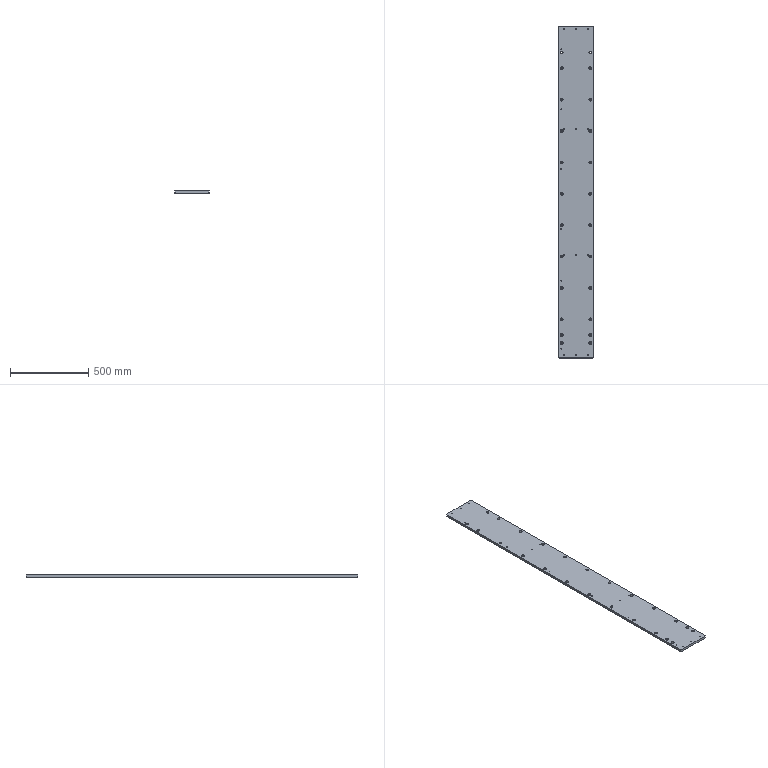Part | SolidWorks | features HoleWzd 3, Chamfer 1, Extrusion 1 | 1 solid | 166 faces | box 220 x 2115 x 15 mm | volume 6896303 mm3 | cylinder 132 | plane 34 | commonest cylinder face diameters 11 x48 18 x48 6.8 x24 5 x12